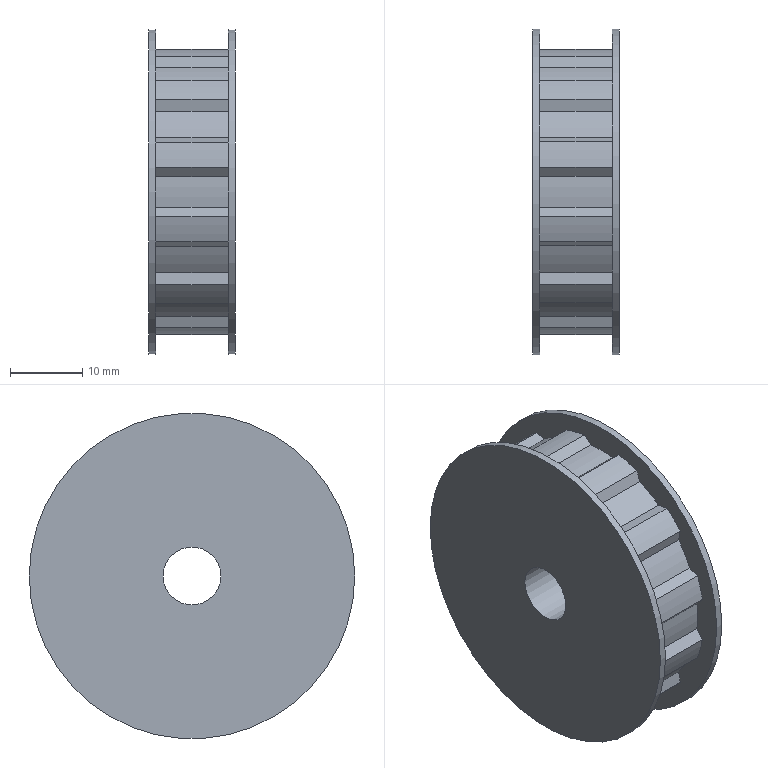Part | NX | features DATUM_CSYS 3, EXTRUDE 2, SKETCH 2, Container 1, EXTRACT_BODY 1, Geometry Instance 1, UNITE 1 | 1 solid | 55 faces | box 12 x 45 x 45 mm | volume 14319 mm3 | plane 28 | cylinder 27 | commonest cylinder face diameters 37.525 x12 40 x12 45 x2 8 x1